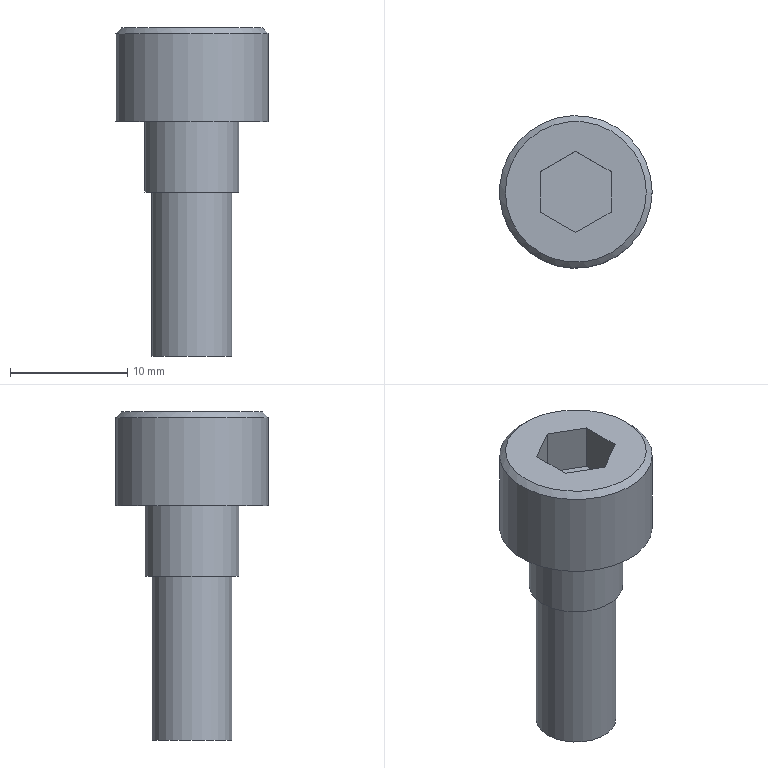Part | STEP file | M3-10_id462_x_t | 1 solid | 15 faces | box 13 x 13 x 28 mm | volume 1742 mm3 | plane 11 | cylinder 3 | cone 1 | commonest cylinder face diameters 6.8 x1 8 x1 13 x1
STEP:
#1=CARTESIAN_POINT('',(-347.4,111.8,-2.));
#2=VERTEX_POINT('',#1);
#3=CARTESIAN_POINT('',(-344.,111.8,-2.));
#4=DIRECTION('',(0.,0.,-1.));
#5=DIRECTION('',(-1.,0.,0.));
#6=AXIS2_PLACEMENT_3D('',#3,#4,#5);
#7=CIRCLE('',#6,3.4);
#8=EDGE_CURVE('',#2,#2,#7,.T.);
#9=ORIENTED_EDGE('',*,*,#8,.F.);
#10=EDGE_LOOP('',(#9));
#11=FACE_BOUND('',#10,.T.);
#12=CARTESIAN_POINT('',(-340.,111.8,-2.));
#13=VERTEX_POINT('',#12);
#14=CARTESIAN_POINT('',(-344.,111.8,-2.));
#15=DIRECTION('',(0.,0.,1.));
#16=DIRECTION('',(1.,0.,0.));
#17=AXIS2_PLACEMENT_3D('',#14,#15,#16);
#18=CIRCLE('',#17,4.);
#19=EDGE_CURVE('',#13,#13,#18,.T.);
#20=ORIENTED_EDGE('',*,*,#19,.F.);
#21=EDGE_LOOP('',(#20));
#22=FACE_BOUND('',#21,.T.);
#23=CARTESIAN_POINT('',(-344.,111.8,-2.));
#24=DIRECTION('',(0.,0.,-1.));
#25=DIRECTION('',(-1.,0.,0.));
#26=AXIS2_PLACEMENT_3D('',#23,#24,#25);
#27=PLANE('',#26);
#28=ADVANCED_FACE('',(#11,#22),#27,.T.);
#29=CARTESIAN_POINT('',(-348.,111.8,4.));
#30=VERTEX_POINT('',#29);
#31=CARTESIAN_POINT('',(-344.,111.8,4.));
#32=DIRECTION('',(0.,0.,1.));
#33=DIRECTION('',(-1.,0.,0.));
#34=AXIS2_PLACEMENT_3D('',#31,#32,#33);
#35=CIRCLE('',#34,4.);
#36=EDGE_CURVE('',#30,#30,#35,.T.);
#37=ORIENTED_EDGE('',*,*,#36,.F.);
#38=EDGE_LOOP('',(#37));
#39=FACE_BOUND('',#38,.T.);
#40=ORIENTED_EDGE('',*,*,#19,.T.);
#41=EDGE_LOOP('',(#40));
#42=FACE_BOUND('',#41,.T.);
#43=CARTESIAN_POINT('',(-344.,111.8,-2.));
#44=DIRECTION('',(0.,0.,1.));
#45=DIRECTION('',(1.,0.,0.));
#46=AXIS2_PLACEMENT_3D('',#43,#44,#45);
#47=CYLINDRICAL_SURFACE('',#46,4.);
#48=ADVANCED_FACE('',(#39,#42),#47,.T.);
#49=CARTESIAN_POINT('',(-340.6,111.8,-16.));
#50=VERTEX_POINT('',#49);
#51=CARTESIAN_POINT('',(-344.,111.8,-16.));
#52=DIRECTION('',(0.,0.,1.));
#53=DIRECTION('',(1.,0.,0.));
#54=AXIS2_PLACEMENT_3D('',#51,#52,#53);
#55=CIRCLE('',#54,3.4);
#56=EDGE_CURVE('',#50,#50,#55,.T.);
#57=ORIENTED_EDGE('',*,*,#56,.F.);
#58=EDGE_LOOP('',(#57));
#59=FACE_OUTER_BOUND('',#58,.T.);
#60=CARTESIAN_POINT('',(-344.,111.8,-16.));
#61=DIRECTION('',(0.,0.,-1.));
#62=DIRECTION('',(-1.,0.,0.));
#63=AXIS2_PLACEMENT_3D('',#60,#61,#62);
#64=PLANE('',#63);
#65=ADVANCED_FACE('',(#59),#64,.T.);
#66=ORIENTED_EDGE('',*,*,#56,.T.);
#67=EDGE_LOOP('',(#66));
#68=FACE_BOUND('',#67,.T.);
#69=ORIENTED_EDGE('',*,*,#8,.T.);
#70=EDGE_LOOP('',(#69));
#71=FACE_BOUND('',#70,.T.);
#72=CARTESIAN_POINT('',(-344.,111.8,-2.));
#73=DIRECTION('',(0.,0.,-1.));
#74=DIRECTION('',(1.,0.,0.));
#75=AXIS2_PLACEMENT_3D('',#72,#73,#74);
#76=CYLINDRICAL_SURFACE('',#75,3.4);
#77=ADVANCED_FACE('',(#68,#71),#76,.T.);
#78=CARTESIAN_POINT('',(-347.,113.532,12.));
#79=VERTEX_POINT('',#78);
#80=CARTESIAN_POINT('',(-347.,110.068,12.));
#81=VERTEX_POINT('',#80);
#82=CARTESIAN_POINT('',(-347.,113.532,12.));
#83=DIRECTION('',(0.,-1.,0.));
#84=VECTOR('',#83,1.);
#85=LINE('',#82,#84);
#86=EDGE_CURVE('',#79,#81,#85,.T.);
#87=ORIENTED_EDGE('',*,*,#86,.F.);
#88=CARTESIAN_POINT('',(-344.,115.264,12.));
#89=VERTEX_POINT('',#88);
#90=CARTESIAN_POINT('',(-344.,115.264,12.));
#91=DIRECTION('',(-0.866,-0.5,0.));
#92=VECTOR('',#91,1.);
#93=LINE('',#90,#92);
#94=EDGE_CURVE('',#89,#79,#93,.T.);
#95=ORIENTED_EDGE('',*,*,#94,.F.);
#96=CARTESIAN_POINT('',(-341.,113.532,12.));
#97=VERTEX_POINT('',#96);
#98=CARTESIAN_POINT('',(-341.,113.532,12.));
#99=DIRECTION('',(-0.866,0.5,0.));
#100=VECTOR('',#99,1.);
#101=LINE('',#98,#100);
#102=EDGE_CURVE('',#97,#89,#101,.T.);
#103=ORIENTED_EDGE('',*,*,#102,.F.);
#104=CARTESIAN_POINT('',(-341.,110.068,12.));
#105=VERTEX_POINT('',#104);
#106=CARTESIAN_POINT('',(-341.,110.068,12.));
#107=DIRECTION('',(0.,1.,0.));
#108=VECTOR('',#107,1.);
#109=LINE('',#106,#108);
#110=EDGE_CURVE('',#105,#97,#109,.T.);
#111=ORIENTED_EDGE('',*,*,#110,.F.);
#112=CARTESIAN_POINT('',(-344.,108.336,12.));
#113=VERTEX_POINT('',#112);
#114=CARTESIAN_POINT('',(-344.,108.336,12.));
#115=DIRECTION('',(0.866,0.5,0.));
#116=VECTOR('',#115,1.);
#117=LINE('',#114,#116);
#118=EDGE_CURVE('',#113,#105,#117,.T.);
#119=ORIENTED_EDGE('',*,*,#118,.F.);
#120=CARTESIAN_POINT('',(-347.,110.068,12.));
#121=DIRECTION('',(0.866,-0.5,0.));
#122=VECTOR('',#121,1.);
#123=LINE('',#120,#122);
#124=EDGE_CURVE('',#81,#113,#123,.T.);
#125=ORIENTED_EDGE('',*,*,#124,.F.);
#126=EDGE_LOOP('',(#87,#95,#103,#111,#119,#125));
#127=FACE_BOUND('',#126,.T.);
#128=CARTESIAN_POINT('',(-338.,111.8,12.));
#129=VERTEX_POINT('',#128);
#130=CARTESIAN_POINT('',(-344.,111.8,12.));
#131=DIRECTION('',(0.,0.,1.));
#132=DIRECTION('',(1.,0.,0.));
#133=AXIS2_PLACEMENT_3D('',#130,#131,#132);
#134=CIRCLE('',#133,6.);
#135=EDGE_CURVE('',#129,#129,#134,.T.);
#136=ORIENTED_EDGE('',*,*,#135,.T.);
#137=EDGE_LOOP('',(#136));
#138=FACE_BOUND('',#137,.T.);
#139=CARTESIAN_POINT('',(-344.,111.8,12.));
#140=DIRECTION('',(0.,0.,1.));
#141=DIRECTION('',(1.,0.,0.));
#142=AXIS2_PLACEMENT_3D('',#139,#140,#141);
#143=PLANE('',#142);
#144=ADVANCED_FACE('',(#127,#138),#143,.T.);
#145=ORIENTED_EDGE('',*,*,#36,.T.);
#146=EDGE_LOOP('',(#145));
#147=FACE_BOUND('',#146,.T.);
#148=CARTESIAN_POINT('',(-337.5,111.8,4.));
#149=VERTEX_POINT('',#148);
#150=CARTESIAN_POINT('',(-344.,111.8,4.));
#151=DIRECTION('',(0.,0.,1.));
#152=DIRECTION('',(1.,0.,0.));
#153=AXIS2_PLACEMENT_3D('',#150,#151,#152);
#154=CIRCLE('',#153,6.5);
#155=EDGE_CURVE('',#149,#149,#154,.T.);
#156=ORIENTED_EDGE('',*,*,#155,.F.);
#157=EDGE_LOOP('',(#156));
#158=FACE_BOUND('',#157,.T.);
#159=CARTESIAN_POINT('',(-344.,111.8,4.));
#160=DIRECTION('',(0.,0.,-1.));
#161=DIRECTION('',(-1.,0.,0.));
#162=AXIS2_PLACEMENT_3D('',#159,#160,#161);
#163=PLANE('',#162);
#164=ADVANCED_FACE('',(#147,#158),#163,.T.);
#165=CARTESIAN_POINT('',(-337.5,111.8,11.5));
#166=VERTEX_POINT('',#165);
#167=CARTESIAN_POINT('',(-344.,111.8,11.5));
#168=DIRECTION('',(0.,0.,-1.));
#169=DIRECTION('',(1.,0.,0.));
#170=AXIS2_PLACEMENT_3D('',#167,#168,#169);
#171=CIRCLE('',#170,6.5);
#172=EDGE_CURVE('',#166,#166,#171,.T.);
#173=ORIENTED_EDGE('',*,*,#172,.T.);
#174=EDGE_LOOP('',(#173));
#175=FACE_BOUND('',#174,.T.);
#176=ORIENTED_EDGE('',*,*,#155,.T.);
#177=EDGE_LOOP('',(#176));
#178=FACE_BOUND('',#177,.T.);
#179=CARTESIAN_POINT('',(-344.,111.8,4.));
#180=DIRECTION('',(0.,0.,1.));
#181=DIRECTION('',(1.,0.,0.));
#182=AXIS2_PLACEMENT_3D('',#179,#180,#181);
#183=CYLINDRICAL_SURFACE('',#182,6.5);
#184=ADVANCED_FACE('',(#175,#178),#183,.T.);
#185=ORIENTED_EDGE('',*,*,#135,.F.);
#186=EDGE_LOOP('',(#185));
#187=FACE_BOUND('',#186,.T.);
#188=ORIENTED_EDGE('',*,*,#172,.F.);
#189=EDGE_LOOP('',(#188));
#190=FACE_BOUND('',#189,.T.);
#191=CARTESIAN_POINT('',(-344.,111.8,11.5));
#192=DIRECTION('',(0.,0.,-1.));
#193=DIRECTION('',(-1.,0.,0.));
#194=AXIS2_PLACEMENT_3D('',#191,#192,#193);
#195=CONICAL_SURFACE('',#194,6.5,45.);
#196=ADVANCED_FACE('',(#187,#190),#195,.T.);
#197=ORIENTED_EDGE('',*,*,#86,.T.);
#198=CARTESIAN_POINT('',(-347.,110.068,8.));
#199=VERTEX_POINT('',#198);
#200=CARTESIAN_POINT('',(-347.,110.068,8.));
#201=DIRECTION('',(0.,0.,-1.));
#202=VECTOR('',#201,1.);
#203=LINE('',#200,#202);
#204=EDGE_CURVE('',#81,#199,#203,.T.);
#205=ORIENTED_EDGE('',*,*,#204,.T.);
#206=CARTESIAN_POINT('',(-347.,113.532,8.));
#207=VERTEX_POINT('',#206);
#208=CARTESIAN_POINT('',(-347.,113.532,8.));
#209=DIRECTION('',(0.,1.,0.));
#210=VECTOR('',#209,1.);
#211=LINE('',#208,#210);
#212=EDGE_CURVE('',#199,#207,#211,.T.);
#213=ORIENTED_EDGE('',*,*,#212,.T.);
#214=CARTESIAN_POINT('',(-347.,113.532,8.));
#215=DIRECTION('',(0.,0.,-1.));
#216=VECTOR('',#215,1.);
#217=LINE('',#214,#216);
#218=EDGE_CURVE('',#79,#207,#217,.T.);
#219=ORIENTED_EDGE('',*,*,#218,.F.);
#220=EDGE_LOOP('',(#197,#205,#213,#219));
#221=FACE_OUTER_BOUND('',#220,.T.);
#222=CARTESIAN_POINT('',(-347.,113.532,8.));
#223=DIRECTION('',(-1.,0.,0.));
#224=DIRECTION('',(0.,-1.,0.));
#225=AXIS2_PLACEMENT_3D('',#222,#223,#224);
#226=PLANE('',#225);
#227=ADVANCED_FACE('',(#221),#226,.F.);
#228=ORIENTED_EDGE('',*,*,#124,.T.);
#229=CARTESIAN_POINT('',(-344.,108.336,8.));
#230=VERTEX_POINT('',#229);
#231=CARTESIAN_POINT('',(-344.,108.336,8.));
#232=DIRECTION('',(0.,0.,-1.));
#233=VECTOR('',#232,1.);
#234=LINE('',#231,#233);
#235=EDGE_CURVE('',#113,#230,#234,.T.);
#236=ORIENTED_EDGE('',*,*,#235,.T.);
#237=CARTESIAN_POINT('',(-347.,110.068,8.));
#238=DIRECTION('',(-0.866,0.5,0.));
#239=VECTOR('',#238,1.);
#240=LINE('',#237,#239);
#241=EDGE_CURVE('',#230,#199,#240,.T.);
#242=ORIENTED_EDGE('',*,*,#241,.T.);
#243=ORIENTED_EDGE('',*,*,#204,.F.);
#244=EDGE_LOOP('',(#228,#236,#242,#243));
#245=FACE_OUTER_BOUND('',#244,.T.);
#246=CARTESIAN_POINT('',(-347.,110.068,8.));
#247=DIRECTION('',(-0.5,-0.866,0.));
#248=DIRECTION('',(0.866,-0.5,0.));
#249=AXIS2_PLACEMENT_3D('',#246,#247,#248);
#250=PLANE('',#249);
#251=ADVANCED_FACE('',(#245),#250,.F.);
#252=ORIENTED_EDGE('',*,*,#118,.T.);
#253=CARTESIAN_POINT('',(-341.,110.068,8.));
#254=VERTEX_POINT('',#253);
#255=CARTESIAN_POINT('',(-341.,110.068,8.));
#256=DIRECTION('',(0.,0.,-1.));
#257=VECTOR('',#256,1.);
#258=LINE('',#255,#257);
#259=EDGE_CURVE('',#105,#254,#258,.T.);
#260=ORIENTED_EDGE('',*,*,#259,.T.);
#261=CARTESIAN_POINT('',(-344.,108.336,8.));
#262=DIRECTION('',(-0.866,-0.5,0.));
#263=VECTOR('',#262,1.);
#264=LINE('',#261,#263);
#265=EDGE_CURVE('',#254,#230,#264,.T.);
#266=ORIENTED_EDGE('',*,*,#265,.T.);
#267=ORIENTED_EDGE('',*,*,#235,.F.);
#268=EDGE_LOOP('',(#252,#260,#266,#267));
#269=FACE_OUTER_BOUND('',#268,.T.);
#270=CARTESIAN_POINT('',(-344.,108.336,8.));
#271=DIRECTION('',(0.5,-0.866,0.));
#272=DIRECTION('',(0.866,0.5,0.));
#273=AXIS2_PLACEMENT_3D('',#270,#271,#272);
#274=PLANE('',#273);
#275=ADVANCED_FACE('',(#269),#274,.F.);
#276=ORIENTED_EDGE('',*,*,#110,.T.);
#277=CARTESIAN_POINT('',(-341.,113.532,8.));
#278=VERTEX_POINT('',#277);
#279=CARTESIAN_POINT('',(-341.,113.532,8.));
#280=DIRECTION('',(0.,0.,-1.));
#281=VECTOR('',#280,1.);
#282=LINE('',#279,#281);
#283=EDGE_CURVE('',#97,#278,#282,.T.);
#284=ORIENTED_EDGE('',*,*,#283,.T.);
#285=CARTESIAN_POINT('',(-341.,110.068,8.));
#286=DIRECTION('',(0.,-1.,0.));
#287=VECTOR('',#286,1.);
#288=LINE('',#285,#287);
#289=EDGE_CURVE('',#278,#254,#288,.T.);
#290=ORIENTED_EDGE('',*,*,#289,.T.);
#291=ORIENTED_EDGE('',*,*,#259,.F.);
#292=EDGE_LOOP('',(#276,#284,#290,#291));
#293=FACE_OUTER_BOUND('',#292,.T.);
#294=CARTESIAN_POINT('',(-341.,110.068,8.));
#295=DIRECTION('',(1.,0.,0.));
#296=DIRECTION('',(0.,1.,0.));
#297=AXIS2_PLACEMENT_3D('',#294,#295,#296);
#298=PLANE('',#297);
#299=ADVANCED_FACE('',(#293),#298,.F.);
#300=ORIENTED_EDGE('',*,*,#102,.T.);
#301=CARTESIAN_POINT('',(-344.,115.264,8.));
#302=VERTEX_POINT('',#301);
#303=CARTESIAN_POINT('',(-344.,115.264,8.));
#304=DIRECTION('',(0.,0.,-1.));
#305=VECTOR('',#304,1.);
#306=LINE('',#303,#305);
#307=EDGE_CURVE('',#89,#302,#306,.T.);
#308=ORIENTED_EDGE('',*,*,#307,.T.);
#309=CARTESIAN_POINT('',(-341.,113.532,8.));
#310=DIRECTION('',(0.866,-0.5,0.));
#311=VECTOR('',#310,1.);
#312=LINE('',#309,#311);
#313=EDGE_CURVE('',#302,#278,#312,.T.);
#314=ORIENTED_EDGE('',*,*,#313,.T.);
#315=ORIENTED_EDGE('',*,*,#283,.F.);
#316=EDGE_LOOP('',(#300,#308,#314,#315));
#317=FACE_OUTER_BOUND('',#316,.T.);
#318=CARTESIAN_POINT('',(-341.,113.532,8.));
#319=DIRECTION('',(0.5,0.866,0.));
#320=DIRECTION('',(-0.866,0.5,0.));
#321=AXIS2_PLACEMENT_3D('',#318,#319,#320);
#322=PLANE('',#321);
#323=ADVANCED_FACE('',(#317),#322,.F.);
#324=ORIENTED_EDGE('',*,*,#94,.T.);
#325=ORIENTED_EDGE('',*,*,#218,.T.);
#326=CARTESIAN_POINT('',(-344.,115.264,8.));
#327=DIRECTION('',(0.866,0.5,0.));
#328=VECTOR('',#327,1.);
#329=LINE('',#326,#328);
#330=EDGE_CURVE('',#207,#302,#329,.T.);
#331=ORIENTED_EDGE('',*,*,#330,.T.);
#332=ORIENTED_EDGE('',*,*,#307,.F.);
#333=EDGE_LOOP('',(#324,#325,#331,#332));
#334=FACE_OUTER_BOUND('',#333,.T.);
#335=CARTESIAN_POINT('',(-344.,115.264,8.));
#336=DIRECTION('',(-0.5,0.866,0.));
#337=DIRECTION('',(-0.866,-0.5,0.));
#338=AXIS2_PLACEMENT_3D('',#335,#336,#337);
#339=PLANE('',#338);
#340=ADVANCED_FACE('',(#334),#339,.F.);
#341=ORIENTED_EDGE('',*,*,#212,.F.);
#342=ORIENTED_EDGE('',*,*,#241,.F.);
#343=ORIENTED_EDGE('',*,*,#265,.F.);
#344=ORIENTED_EDGE('',*,*,#289,.F.);
#345=ORIENTED_EDGE('',*,*,#313,.F.);
#346=ORIENTED_EDGE('',*,*,#330,.F.);
#347=EDGE_LOOP('',(#341,#342,#343,#344,#345,#346));
#348=FACE_OUTER_BOUND('',#347,.T.);
#349=CARTESIAN_POINT('',(-344.,111.8,8.));
#350=DIRECTION('',(0.,0.,1.));
#351=DIRECTION('',(1.,0.,0.));
#352=AXIS2_PLACEMENT_3D('',#349,#350,#351);
#353=PLANE('',#352);
#354=ADVANCED_FACE('',(#348),#353,.T.);
#355=CLOSED_SHELL('',(#28,#48,#65,#77,#144,#164,#184,#196,#227,#251,#275,#299,#323,#340,#354));
#356=MANIFOLD_SOLID_BREP('',#355);
#357=(LENGTH_UNIT()NAMED_UNIT(*)SI_UNIT(.MILLI.,.METRE.));
#358=UNCERTAINTY_MEASURE_WITH_UNIT(LENGTH_MEASURE(0.00002),#357,'','');
#359=(NAMED_UNIT(*)PLANE_ANGLE_UNIT()SI_UNIT($,.RADIAN.));
#360=PLANE_ANGLE_MEASURE_WITH_UNIT(PLANE_ANGLE_MEASURE(0.01745),#359);
#361=DIMENSIONAL_EXPONENTS(0.,0.,0.,0.,0.,0.,0.);
#362=(CONVERSION_BASED_UNIT('DEGREE',#360)NAMED_UNIT(#361)PLANE_ANGLE_UNIT());
#363=(NAMED_UNIT(*)SI_UNIT($,.STERADIAN.)SOLID_ANGLE_UNIT());
#364=(GEOMETRIC_REPRESENTATION_CONTEXT(3)GLOBAL_UNCERTAINTY_ASSIGNED_CONTEXT((#358))GLOBAL_UNIT_ASSIGNED_CONTEXT((#357,#362,#363))REPRESENTATION_CONTEXT('',''));
#365=ADVANCED_BREP_SHAPE_REPRESENTATION('',(#356),#364);